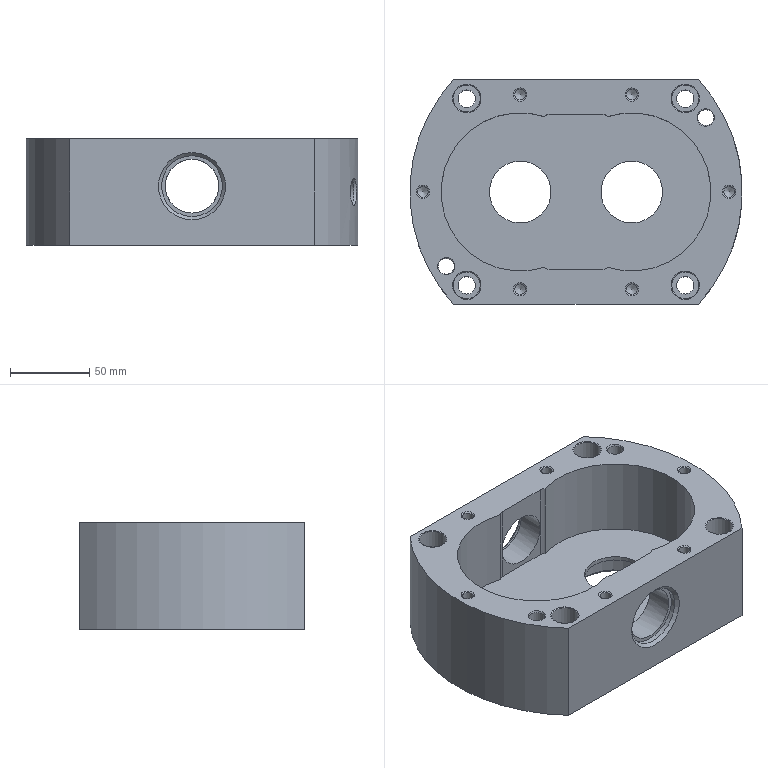Part | 1 solid | 233 faces | box 210 x 142 x 67.4 mm | volume 724642 mm3 | cylinder 120 | plane 71 | cone 40 | spline 2 | commonest cylinder face diameters 8 x58 114 x9 4.2 x8 6.8 x6 11 x4 17 x4